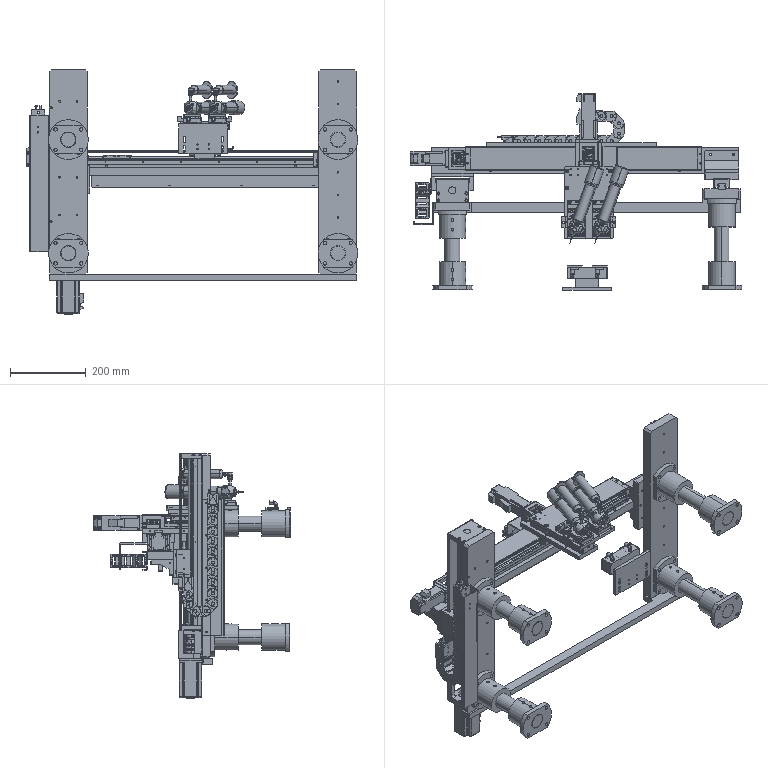Part | NX | features BREP 77 | 139 solids | 8377 faces | volume 12968592 mm3 | plane 4111 | cylinder 3466 | cone 604 | torus 116 | sphere 48 | spline 32 | commonest cylinder face diameters 8 x311 3.3 x216 3 x194 2.5 x182 4.5 x182 6 x153